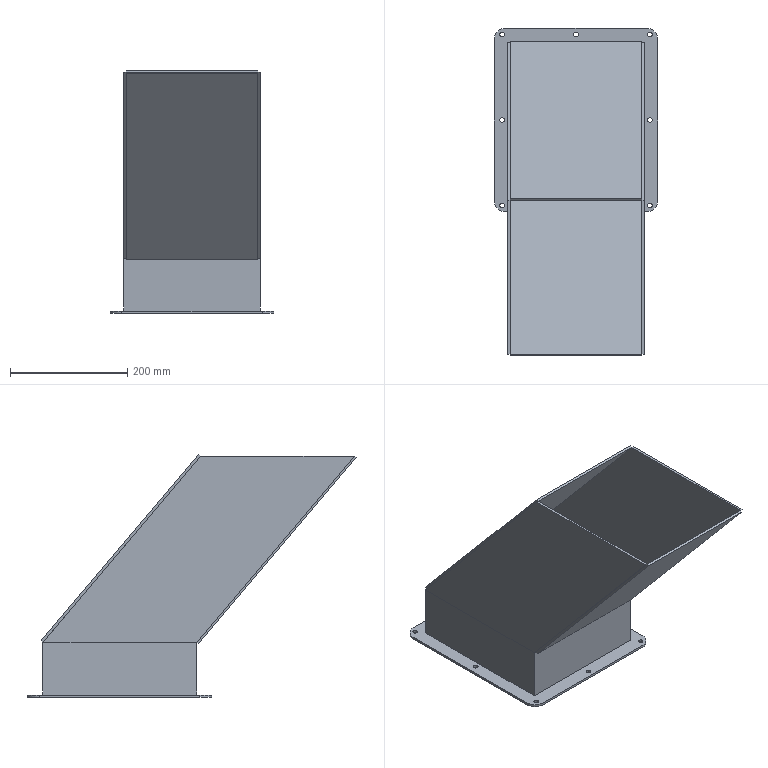Part | STEP file | odciag11V11 | 5 solids | 59 faces | box 280 x 560.788 x 414.862 mm | volume 1890664 mm3 | plane 39 | cylinder 20 | commonest cylinder face diameters 8 x16 40 x4